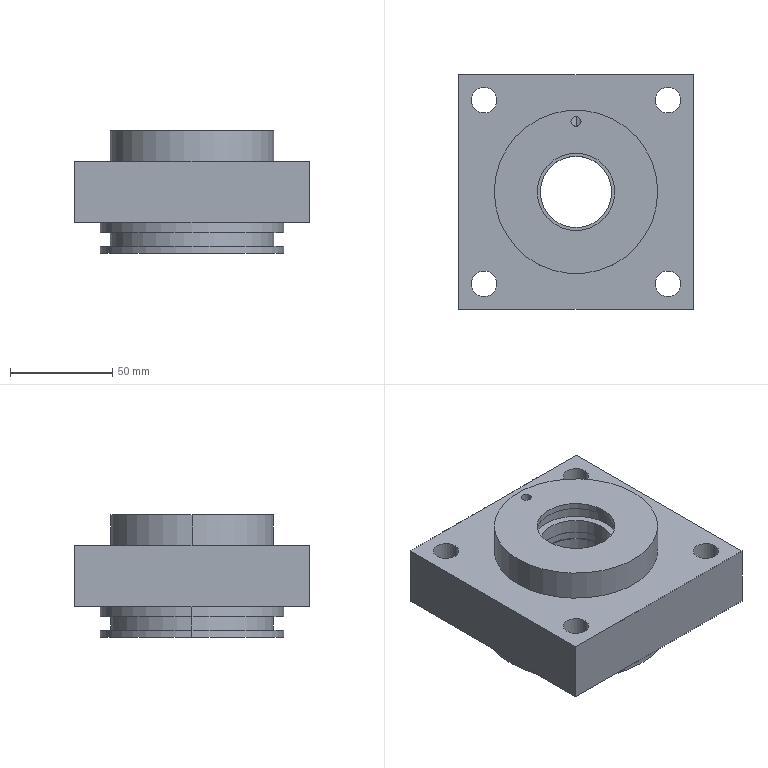Part | SolidWorks | features ICE 4, Extrusion 1, HoleWzd 1, RevCut 1 | 1 solid | 71 faces | box 115 x 115 x 60 mm | volume 477464 mm3 | cylinder 44 | plane 23 | cone 4 | commonest cylinder face diameters 12.5 x8 35 x8 36 x6 38 x4 80 x4 90 x4